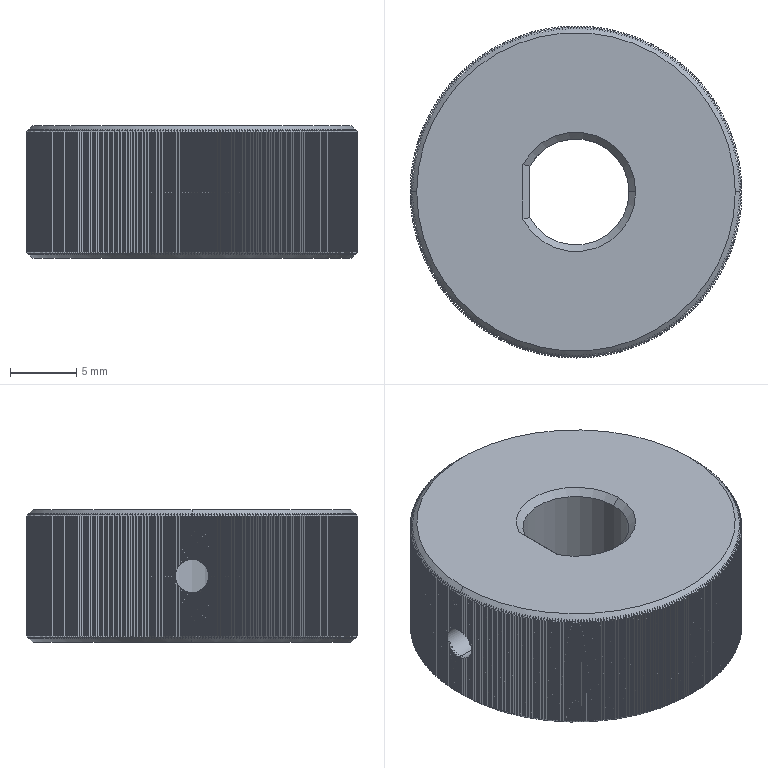Part | NX | features BREP 1 | 1 solid | 1129 faces | box 25 x 25 x 10 mm | volume 4302 mm3 | plane 748 | cylinder 374 | cone 7 | commonest cylinder face diameters 25 x371 2.5 x2 8 x1